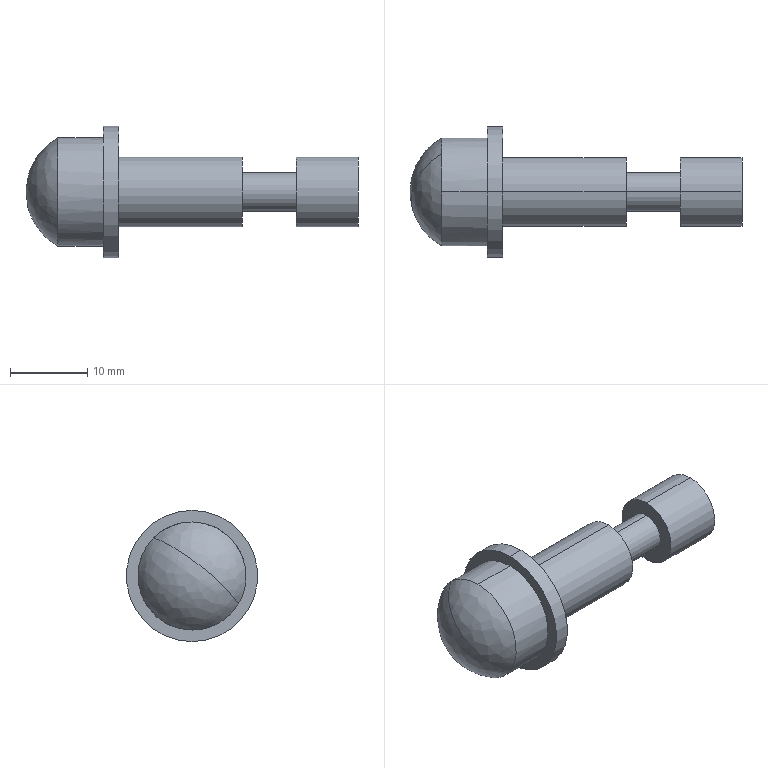Part | SolidWorks | features BaseBody 1 | 1 solid | 17 faces | box 43 x 17 x 17 mm | volume 3377 mm3 | cylinder 10 | plane 5 | spline 2 | commonest cylinder face diameters 9 x4 5 x2 14 x2 17 x2
STEP:
#1=CARTESIAN_POINT('',(867.073,-4291.009,964.907));
#2=VERTEX_POINT('',#1);
#3=CARTESIAN_POINT('',(867.073,-4295.973,966.971));
#4=VERTEX_POINT('',#3);
#5=CARTESIAN_POINT('',(867.073,-4295.973,959.971));
#6=DIRECTION('',(1.,0.,0.));
#7=DIRECTION('',(0.,0.,-1.));
#8=AXIS2_PLACEMENT_3D('',#5,#6,#7);
#9=CIRCLE('',#8,7.);
#10=EDGE_CURVE('',#2,#4,#9,.T.);
#11=ORIENTED_EDGE('',*,*,#10,.F.);
#12=CARTESIAN_POINT('',(867.073,-4301.97,956.36));
#13=VERTEX_POINT('',#12);
#14=CARTESIAN_POINT('',(870.946,-4295.973,959.971));
#15=DIRECTION('',(0.2119,-0.6009,0.7707));
#16=DIRECTION('',(0.1555,0.7993,0.5805));
#17=AXIS2_PLACEMENT_3D('',#14,#15,#16);
#18=CIRCLE('',#17,8.);
#19=EDGE_CURVE('',#2,#13,#18,.T.);
#20=ORIENTED_EDGE('',*,*,#19,.T.);
#21=CARTESIAN_POINT('',(867.073,-4295.973,959.971));
#22=DIRECTION('',(1.,0.,0.));
#23=DIRECTION('',(0.,0.,-1.));
#24=AXIS2_PLACEMENT_3D('',#21,#22,#23);
#25=CIRCLE('',#24,7.);
#26=EDGE_CURVE('',#4,#13,#25,.T.);
#27=ORIENTED_EDGE('',*,*,#26,.F.);
#28=EDGE_LOOP('',(#11,#20,#27));
#29=FACE_OUTER_BOUND('',#28,.T.);
#30=CARTESIAN_POINT('',(867.159,-4290.959,964.923));
#31=CARTESIAN_POINT('',(867.476,-4291.86,966.078));
#32=CARTESIAN_POINT('',(868.38,-4292.673,966.955));
#33=CARTESIAN_POINT('',(869.698,-4293.242,967.387));
#34=CARTESIAN_POINT('',(861.079,-4294.485,963.844));
#35=CARTESIAN_POINT('',(861.757,-4296.406,966.308));
#36=CARTESIAN_POINT('',(863.685,-4298.14,968.179));
#37=CARTESIAN_POINT('',(866.495,-4299.355,969.099));
#38=CARTESIAN_POINT('',(861.079,-4300.092,959.472));
#39=CARTESIAN_POINT('',(861.684,-4301.807,961.672));
#40=CARTESIAN_POINT('',(863.405,-4303.354,963.341));
#41=CARTESIAN_POINT('',(865.913,-4304.439,964.163));
#42=CARTESIAN_POINT('',(867.159,-4301.997,956.315));
#43=CARTESIAN_POINT('',(867.333,-4302.492,956.95));
#44=CARTESIAN_POINT('',(867.829,-4302.938,957.431));
#45=CARTESIAN_POINT('',(868.553,-4303.251,957.668));
#46=(BOUNDED_SURFACE()B_SPLINE_SURFACE(3,3,((#30,#31,#32,#33),(#34,#35,#36,#37),(#38,#39,#40,#41),(#42,#43,#44,#45)),.UNSPECIFIED.,.F.,.F.,.T.)B_SPLINE_SURFACE_WITH_KNOTS((4,4),(4,4),(0.,1.),(0.,1.),.UNSPECIFIED.)GEOMETRIC_REPRESENTATION_ITEM()RATIONAL_B_SPLINE_SURFACE(((1.,0.9364,0.9364,1.),(0.6562,0.6145,0.6145,0.6562),(0.6562,0.6145,0.6145,0.6562),(1.,0.9364,0.9364,1.)))REPRESENTATION_ITEM('')SURFACE());
#47=ADVANCED_FACE('',(#29),#46,.T.);
#48=CARTESIAN_POINT('',(874.946,-4295.973,955.471));
#49=VERTEX_POINT('',#48);
#50=CARTESIAN_POINT('',(874.946,-4295.973,964.471));
#51=VERTEX_POINT('',#50);
#52=CARTESIAN_POINT('',(874.946,-4295.973,959.971));
#53=DIRECTION('',(1.,0.,0.));
#54=DIRECTION('',(0.,0.,-1.));
#55=AXIS2_PLACEMENT_3D('',#52,#53,#54);
#56=CIRCLE('',#55,4.5);
#57=EDGE_CURVE('',#49,#51,#56,.T.);
#58=ORIENTED_EDGE('',*,*,#57,.T.);
#59=CARTESIAN_POINT('',(890.946,-4295.973,964.471));
#60=VERTEX_POINT('',#59);
#61=CARTESIAN_POINT('',(880.946,-4295.973,964.471));
#62=DIRECTION('',(1.,0.,0.));
#63=VECTOR('',#62,1000.);
#64=LINE('',#61,#63);
#65=EDGE_CURVE('',#51,#60,#64,.T.);
#66=ORIENTED_EDGE('',*,*,#65,.T.);
#67=CARTESIAN_POINT('',(890.946,-4295.973,955.471));
#68=VERTEX_POINT('',#67);
#69=CARTESIAN_POINT('',(890.946,-4295.973,959.971));
#70=DIRECTION('',(-1.,0.,0.));
#71=DIRECTION('',(0.,0.,-1.));
#72=AXIS2_PLACEMENT_3D('',#69,#70,#71);
#73=CIRCLE('',#72,4.5);
#74=EDGE_CURVE('',#60,#68,#73,.T.);
#75=ORIENTED_EDGE('',*,*,#74,.T.);
#76=CARTESIAN_POINT('',(880.946,-4295.973,955.471));
#77=DIRECTION('',(1.,0.,0.));
#78=VECTOR('',#77,1000.);
#79=LINE('',#76,#78);
#80=EDGE_CURVE('',#49,#68,#79,.T.);
#81=ORIENTED_EDGE('',*,*,#80,.F.);
#82=EDGE_LOOP('',(#58,#66,#75,#81));
#83=FACE_OUTER_BOUND('',#82,.T.);
#84=CARTESIAN_POINT('',(880.946,-4295.973,959.971));
#85=DIRECTION('',(1.,0.,0.));
#86=DIRECTION('',(0.,0.,-1.));
#87=AXIS2_PLACEMENT_3D('',#84,#85,#86);
#88=CYLINDRICAL_SURFACE('',#87,4.5);
#89=ADVANCED_FACE('',(#83),#88,.T.);
#90=CARTESIAN_POINT('',(890.946,-4295.973,962.471));
#91=VERTEX_POINT('',#90);
#92=CARTESIAN_POINT('',(890.946,-4295.973,957.471));
#93=VERTEX_POINT('',#92);
#94=CARTESIAN_POINT('',(890.946,-4295.973,959.971));
#95=DIRECTION('',(-1.,0.,0.));
#96=DIRECTION('',(0.,0.,-1.));
#97=AXIS2_PLACEMENT_3D('',#94,#95,#96);
#98=CIRCLE('',#97,2.5);
#99=EDGE_CURVE('',#91,#93,#98,.T.);
#100=ORIENTED_EDGE('',*,*,#99,.F.);
#101=CARTESIAN_POINT('',(897.946,-4295.973,962.471));
#102=VERTEX_POINT('',#101);
#103=CARTESIAN_POINT('',(892.446,-4295.973,962.471));
#104=DIRECTION('',(1.,0.,0.));
#105=VECTOR('',#104,1000.);
#106=LINE('',#103,#105);
#107=EDGE_CURVE('',#91,#102,#106,.T.);
#108=ORIENTED_EDGE('',*,*,#107,.T.);
#109=CARTESIAN_POINT('',(897.946,-4295.973,957.471));
#110=VERTEX_POINT('',#109);
#111=CARTESIAN_POINT('',(897.946,-4295.973,959.971));
#112=DIRECTION('',(-1.,0.,0.));
#113=DIRECTION('',(0.,0.,-1.));
#114=AXIS2_PLACEMENT_3D('',#111,#112,#113);
#115=CIRCLE('',#114,2.5);
#116=EDGE_CURVE('',#102,#110,#115,.T.);
#117=ORIENTED_EDGE('',*,*,#116,.T.);
#118=CARTESIAN_POINT('',(892.446,-4295.973,957.471));
#119=DIRECTION('',(1.,0.,0.));
#120=VECTOR('',#119,1000.);
#121=LINE('',#118,#120);
#122=EDGE_CURVE('',#93,#110,#121,.T.);
#123=ORIENTED_EDGE('',*,*,#122,.F.);
#124=EDGE_LOOP('',(#100,#108,#117,#123));
#125=FACE_OUTER_BOUND('',#124,.T.);
#126=CARTESIAN_POINT('',(892.446,-4295.973,959.971));
#127=DIRECTION('',(1.,0.,0.));
#128=DIRECTION('',(0.,0.,-1.));
#129=AXIS2_PLACEMENT_3D('',#126,#127,#128);
#130=CYLINDRICAL_SURFACE('',#129,2.5);
#131=ADVANCED_FACE('',(#125),#130,.T.);
#132=CARTESIAN_POINT('',(872.946,-4295.973,951.471));
#133=VERTEX_POINT('',#132);
#134=CARTESIAN_POINT('',(872.946,-4295.973,968.471));
#135=VERTEX_POINT('',#134);
#136=CARTESIAN_POINT('',(872.946,-4295.973,959.971));
#137=DIRECTION('',(1.,0.,0.));
#138=DIRECTION('',(0.,0.,-1.));
#139=AXIS2_PLACEMENT_3D('',#136,#137,#138);
#140=CIRCLE('',#139,8.5);
#141=EDGE_CURVE('',#133,#135,#140,.T.);
#142=ORIENTED_EDGE('',*,*,#141,.T.);
#143=CARTESIAN_POINT('',(874.946,-4295.973,968.471));
#144=VERTEX_POINT('',#143);
#145=CARTESIAN_POINT('',(871.946,-4295.973,968.471));
#146=DIRECTION('',(1.,0.,0.));
#147=VECTOR('',#146,1000.);
#148=LINE('',#145,#147);
#149=EDGE_CURVE('',#135,#144,#148,.T.);
#150=ORIENTED_EDGE('',*,*,#149,.T.);
#151=CARTESIAN_POINT('',(874.946,-4295.973,951.471));
#152=VERTEX_POINT('',#151);
#153=CARTESIAN_POINT('',(874.946,-4295.973,959.971));
#154=DIRECTION('',(1.,0.,0.));
#155=DIRECTION('',(0.,0.,-1.));
#156=AXIS2_PLACEMENT_3D('',#153,#154,#155);
#157=CIRCLE('',#156,8.5);
#158=EDGE_CURVE('',#152,#144,#157,.T.);
#159=ORIENTED_EDGE('',*,*,#158,.F.);
#160=CARTESIAN_POINT('',(871.946,-4295.973,951.471));
#161=DIRECTION('',(1.,0.,0.));
#162=VECTOR('',#161,1000.);
#163=LINE('',#160,#162);
#164=EDGE_CURVE('',#133,#152,#163,.T.);
#165=ORIENTED_EDGE('',*,*,#164,.F.);
#166=EDGE_LOOP('',(#142,#150,#159,#165));
#167=FACE_OUTER_BOUND('',#166,.T.);
#168=CARTESIAN_POINT('',(871.946,-4295.973,959.971));
#169=DIRECTION('',(1.,0.,0.));
#170=DIRECTION('',(0.,0.,-1.));
#171=AXIS2_PLACEMENT_3D('',#168,#169,#170);
#172=CYLINDRICAL_SURFACE('',#171,8.5);
#173=ADVANCED_FACE('',(#167),#172,.T.);
#174=CARTESIAN_POINT('',(897.946,-4295.973,964.471));
#175=VERTEX_POINT('',#174);
#176=CARTESIAN_POINT('',(897.946,-4295.973,955.471));
#177=VERTEX_POINT('',#176);
#178=CARTESIAN_POINT('',(897.946,-4295.973,959.971));
#179=DIRECTION('',(-1.,0.,0.));
#180=DIRECTION('',(0.,0.,-1.));
#181=AXIS2_PLACEMENT_3D('',#178,#179,#180);
#182=CIRCLE('',#181,4.5);
#183=EDGE_CURVE('',#175,#177,#182,.T.);
#184=ORIENTED_EDGE('',*,*,#183,.F.);
#185=CARTESIAN_POINT('',(905.946,-4295.973,964.471));
#186=VERTEX_POINT('',#185);
#187=CARTESIAN_POINT('',(899.946,-4295.973,964.471));
#188=DIRECTION('',(1.,0.,0.));
#189=VECTOR('',#188,1000.);
#190=LINE('',#187,#189);
#191=EDGE_CURVE('',#175,#186,#190,.T.);
#192=ORIENTED_EDGE('',*,*,#191,.T.);
#193=CARTESIAN_POINT('',(905.946,-4295.973,955.471));
#194=VERTEX_POINT('',#193);
#195=CARTESIAN_POINT('',(905.946,-4295.973,959.971));
#196=DIRECTION('',(-1.,0.,0.));
#197=DIRECTION('',(0.,0.,-1.));
#198=AXIS2_PLACEMENT_3D('',#195,#196,#197);
#199=CIRCLE('',#198,4.5);
#200=EDGE_CURVE('',#186,#194,#199,.T.);
#201=ORIENTED_EDGE('',*,*,#200,.T.);
#202=CARTESIAN_POINT('',(899.946,-4295.973,955.471));
#203=DIRECTION('',(1.,0.,0.));
#204=VECTOR('',#203,1000.);
#205=LINE('',#202,#204);
#206=EDGE_CURVE('',#177,#194,#205,.T.);
#207=ORIENTED_EDGE('',*,*,#206,.F.);
#208=EDGE_LOOP('',(#184,#192,#201,#207));
#209=FACE_OUTER_BOUND('',#208,.T.);
#210=CARTESIAN_POINT('',(899.946,-4295.973,959.971));
#211=DIRECTION('',(1.,0.,0.));
#212=DIRECTION('',(0.,0.,-1.));
#213=AXIS2_PLACEMENT_3D('',#210,#211,#212);
#214=CYLINDRICAL_SURFACE('',#213,4.5);
#215=ADVANCED_FACE('',(#209),#214,.T.);
#216=CARTESIAN_POINT('',(867.073,-4295.973,952.971));
#217=VERTEX_POINT('',#216);
#218=CARTESIAN_POINT('',(867.073,-4295.973,959.971));
#219=DIRECTION('',(1.,0.,0.));
#220=DIRECTION('',(0.,0.,-1.));
#221=AXIS2_PLACEMENT_3D('',#218,#219,#220);
#222=CIRCLE('',#221,7.);
#223=EDGE_CURVE('',#217,#2,#222,.T.);
#224=ORIENTED_EDGE('',*,*,#223,.T.);
#225=ORIENTED_EDGE('',*,*,#10,.T.);
#226=CARTESIAN_POINT('',(872.946,-4295.973,966.971));
#227=VERTEX_POINT('',#226);
#228=CARTESIAN_POINT('',(869.009,-4295.973,966.971));
#229=DIRECTION('',(1.,0.,0.));
#230=VECTOR('',#229,1000.);
#231=LINE('',#228,#230);
#232=EDGE_CURVE('',#4,#227,#231,.T.);
#233=ORIENTED_EDGE('',*,*,#232,.T.);
#234=CARTESIAN_POINT('',(872.946,-4295.973,952.971));
#235=VERTEX_POINT('',#234);
#236=CARTESIAN_POINT('',(872.946,-4295.973,959.971));
#237=DIRECTION('',(1.,0.,0.));
#238=DIRECTION('',(0.,0.,-1.));
#239=AXIS2_PLACEMENT_3D('',#236,#237,#238);
#240=CIRCLE('',#239,7.);
#241=EDGE_CURVE('',#235,#227,#240,.T.);
#242=ORIENTED_EDGE('',*,*,#241,.F.);
#243=CARTESIAN_POINT('',(869.009,-4295.973,952.971));
#244=DIRECTION('',(1.,0.,0.));
#245=VECTOR('',#244,1000.);
#246=LINE('',#243,#245);
#247=EDGE_CURVE('',#217,#235,#246,.T.);
#248=ORIENTED_EDGE('',*,*,#247,.F.);
#249=EDGE_LOOP('',(#224,#225,#233,#242,#248));
#250=FACE_OUTER_BOUND('',#249,.T.);
#251=CARTESIAN_POINT('',(869.009,-4295.973,959.971));
#252=DIRECTION('',(1.,0.,0.));
#253=DIRECTION('',(0.,0.,-1.));
#254=AXIS2_PLACEMENT_3D('',#251,#252,#253);
#255=CYLINDRICAL_SURFACE('',#254,7.);
#256=ADVANCED_FACE('',(#250),#255,.T.);
#257=ORIENTED_EDGE('',*,*,#65,.F.);
#258=CARTESIAN_POINT('',(874.946,-4295.973,959.971));
#259=DIRECTION('',(1.,0.,0.));
#260=DIRECTION('',(0.,0.,-1.));
#261=AXIS2_PLACEMENT_3D('',#258,#259,#260);
#262=CIRCLE('',#261,4.5);
#263=EDGE_CURVE('',#51,#49,#262,.T.);
#264=ORIENTED_EDGE('',*,*,#263,.T.);
#265=ORIENTED_EDGE('',*,*,#80,.T.);
#266=CARTESIAN_POINT('',(890.946,-4295.973,959.971));
#267=DIRECTION('',(-1.,0.,0.));
#268=DIRECTION('',(0.,0.,-1.));
#269=AXIS2_PLACEMENT_3D('',#266,#267,#268);
#270=CIRCLE('',#269,4.5);
#271=EDGE_CURVE('',#68,#60,#270,.T.);
#272=ORIENTED_EDGE('',*,*,#271,.T.);
#273=EDGE_LOOP('',(#257,#264,#265,#272));
#274=FACE_OUTER_BOUND('',#273,.T.);
#275=CARTESIAN_POINT('',(880.946,-4295.973,959.971));
#276=DIRECTION('',(1.,0.,0.));
#277=DIRECTION('',(0.,0.,-1.));
#278=AXIS2_PLACEMENT_3D('',#275,#276,#277);
#279=CYLINDRICAL_SURFACE('',#278,4.5);
#280=ADVANCED_FACE('',(#274),#279,.T.);
#281=ORIENTED_EDGE('',*,*,#271,.F.);
#282=ORIENTED_EDGE('',*,*,#74,.F.);
#283=EDGE_LOOP('',(#281,#282));
#284=FACE_OUTER_BOUND('',#283,.T.);
#285=CARTESIAN_POINT('',(890.946,-4295.973,959.971));
#286=DIRECTION('',(-1.,0.,0.));
#287=DIRECTION('',(0.,0.,-1.));
#288=AXIS2_PLACEMENT_3D('',#285,#286,#287);
#289=CIRCLE('',#288,2.5);
#290=EDGE_CURVE('',#93,#91,#289,.T.);
#291=ORIENTED_EDGE('',*,*,#290,.T.);
#292=ORIENTED_EDGE('',*,*,#99,.T.);
#293=EDGE_LOOP('',(#291,#292));
#294=FACE_BOUND('',#293,.T.);
#295=CARTESIAN_POINT('',(890.946,-4292.473,959.971));
#296=DIRECTION('',(1.,0.,0.));
#297=DIRECTION('',(0.,0.,-1.));
#298=AXIS2_PLACEMENT_3D('',#295,#296,#297);
#299=PLANE('',#298);
#300=ADVANCED_FACE('',(#284,#294),#299,.T.);
#301=ORIENTED_EDGE('',*,*,#158,.T.);
#302=CARTESIAN_POINT('',(874.946,-4295.973,959.971));
#303=DIRECTION('',(1.,0.,0.));
#304=DIRECTION('',(0.,0.,-1.));
#305=AXIS2_PLACEMENT_3D('',#302,#303,#304);
#306=CIRCLE('',#305,8.5);
#307=EDGE_CURVE('',#144,#152,#306,.T.);
#308=ORIENTED_EDGE('',*,*,#307,.T.);
#309=EDGE_LOOP('',(#301,#308));
#310=FACE_OUTER_BOUND('',#309,.T.);
#311=ORIENTED_EDGE('',*,*,#57,.F.);
#312=ORIENTED_EDGE('',*,*,#263,.F.);
#313=EDGE_LOOP('',(#311,#312));
#314=FACE_BOUND('',#313,.T.);
#315=CARTESIAN_POINT('',(874.946,-4289.473,959.971));
#316=DIRECTION('',(1.,0.,0.));
#317=DIRECTION('',(0.,0.,-1.));
#318=AXIS2_PLACEMENT_3D('',#315,#316,#317);
#319=PLANE('',#318);
#320=ADVANCED_FACE('',(#310,#314),#319,.T.);
#321=ORIENTED_EDGE('',*,*,#107,.F.);
#322=ORIENTED_EDGE('',*,*,#290,.F.);
#323=ORIENTED_EDGE('',*,*,#122,.T.);
#324=CARTESIAN_POINT('',(897.946,-4295.973,959.971));
#325=DIRECTION('',(-1.,0.,0.));
#326=DIRECTION('',(0.,0.,-1.));
#327=AXIS2_PLACEMENT_3D('',#324,#325,#326);
#328=CIRCLE('',#327,2.5);
#329=EDGE_CURVE('',#110,#102,#328,.T.);
#330=ORIENTED_EDGE('',*,*,#329,.T.);
#331=EDGE_LOOP('',(#321,#322,#323,#330));
#332=FACE_OUTER_BOUND('',#331,.T.);
#333=CARTESIAN_POINT('',(892.446,-4295.973,959.971));
#334=DIRECTION('',(1.,0.,0.));
#335=DIRECTION('',(0.,0.,-1.));
#336=AXIS2_PLACEMENT_3D('',#333,#334,#335);
#337=CYLINDRICAL_SURFACE('',#336,2.5);
#338=ADVANCED_FACE('',(#332),#337,.T.);
#339=ORIENTED_EDGE('',*,*,#149,.F.);
#340=CARTESIAN_POINT('',(872.946,-4295.973,959.971));
#341=DIRECTION('',(1.,0.,0.));
#342=DIRECTION('',(0.,0.,-1.));
#343=AXIS2_PLACEMENT_3D('',#340,#341,#342);
#344=CIRCLE('',#343,8.5);
#345=EDGE_CURVE('',#135,#133,#344,.T.);
#346=ORIENTED_EDGE('',*,*,#345,.T.);
#347=ORIENTED_EDGE('',*,*,#164,.T.);
#348=ORIENTED_EDGE('',*,*,#307,.F.);
#349=EDGE_LOOP('',(#339,#346,#347,#348));
#350=FACE_OUTER_BOUND('',#349,.T.);
#351=CARTESIAN_POINT('',(871.946,-4295.973,959.971));
#352=DIRECTION('',(1.,0.,0.));
#353=DIRECTION('',(0.,0.,-1.));
#354=AXIS2_PLACEMENT_3D('',#351,#352,#353);
#355=CYLINDRICAL_SURFACE('',#354,8.5);
#356=ADVANCED_FACE('',(#350),#355,.T.);
#357=ORIENTED_EDGE('',*,*,#329,.F.);
#358=ORIENTED_EDGE('',*,*,#116,.F.);
#359=EDGE_LOOP('',(#357,#358));
#360=FACE_BOUND('',#359,.T.);
#361=CARTESIAN_POINT('',(897.946,-4295.973,959.971));
#362=DIRECTION('',(-1.,0.,0.));
#363=DIRECTION('',(0.,0.,-1.));
#364=AXIS2_PLACEMENT_3D('',#361,#362,#363);
#365=CIRCLE('',#364,4.5);
#366=EDGE_CURVE('',#177,#175,#365,.T.);
#367=ORIENTED_EDGE('',*,*,#366,.T.);
#368=ORIENTED_EDGE('',*,*,#183,.T.);
#369=EDGE_LOOP('',(#367,#368));
#370=FACE_OUTER_BOUND('',#369,.T.);
#371=CARTESIAN_POINT('',(897.946,-4292.473,959.971));
#372=DIRECTION('',(-1.,0.,0.));
#373=DIRECTION('',(0.,0.,1.));
#374=AXIS2_PLACEMENT_3D('',#371,#372,#373);
#375=PLANE('',#374);
#376=ADVANCED_FACE('',(#360,#370),#375,.T.);
#377=ORIENTED_EDGE('',*,*,#241,.T.);
#378=CARTESIAN_POINT('',(872.946,-4295.973,959.971));
#379=DIRECTION('',(1.,0.,0.));
#380=DIRECTION('',(0.,0.,-1.));
#381=AXIS2_PLACEMENT_3D('',#378,#379,#380);
#382=CIRCLE('',#381,7.);
#383=EDGE_CURVE('',#227,#235,#382,.T.);
#384=ORIENTED_EDGE('',*,*,#383,.T.);
#385=EDGE_LOOP('',(#377,#384));
#386=FACE_BOUND('',#385,.T.);
#387=ORIENTED_EDGE('',*,*,#141,.F.);
#388=ORIENTED_EDGE('',*,*,#345,.F.);
#389=EDGE_LOOP('',(#387,#388));
#390=FACE_OUTER_BOUND('',#389,.T.);
#391=CARTESIAN_POINT('',(872.946,-4288.223,959.971));
#392=DIRECTION('',(-1.,0.,0.));
#393=DIRECTION('',(0.,0.,1.));
#394=AXIS2_PLACEMENT_3D('',#391,#392,#393);
#395=PLANE('',#394);
#396=ADVANCED_FACE('',(#386,#390),#395,.T.);
#397=ORIENTED_EDGE('',*,*,#191,.F.);
#398=ORIENTED_EDGE('',*,*,#366,.F.);
#399=ORIENTED_EDGE('',*,*,#206,.T.);
#400=CARTESIAN_POINT('',(905.946,-4295.973,959.971));
#401=DIRECTION('',(-1.,0.,0.));
#402=DIRECTION('',(0.,0.,-1.));
#403=AXIS2_PLACEMENT_3D('',#400,#401,#402);
#404=CIRCLE('',#403,4.5);
#405=EDGE_CURVE('',#194,#186,#404,.T.);
#406=ORIENTED_EDGE('',*,*,#405,.T.);
#407=EDGE_LOOP('',(#397,#398,#399,#406));
#408=FACE_OUTER_BOUND('',#407,.T.);
#409=CARTESIAN_POINT('',(899.946,-4295.973,959.971));
#410=DIRECTION('',(1.,0.,0.));
#411=DIRECTION('',(0.,0.,-1.));
#412=AXIS2_PLACEMENT_3D('',#409,#410,#411);
#413=CYLINDRICAL_SURFACE('',#412,4.5);
#414=ADVANCED_FACE('',(#408),#413,.T.);
#415=ORIENTED_EDGE('',*,*,#232,.F.);
#416=ORIENTED_EDGE('',*,*,#26,.T.);
#417=CARTESIAN_POINT('',(867.073,-4295.973,959.971));
#418=DIRECTION('',(1.,0.,0.));
#419=DIRECTION('',(0.,0.,-1.));
#420=AXIS2_PLACEMENT_3D('',#417,#418,#419);
#421=CIRCLE('',#420,7.);
#422=EDGE_CURVE('',#13,#217,#421,.T.);
#423=ORIENTED_EDGE('',*,*,#422,.T.);
#424=ORIENTED_EDGE('',*,*,#247,.T.);
#425=ORIENTED_EDGE('',*,*,#383,.F.);
#426=EDGE_LOOP('',(#415,#416,#423,#424,#425));
#427=FACE_OUTER_BOUND('',#426,.T.);
#428=CARTESIAN_POINT('',(869.009,-4295.973,959.971));
#429=DIRECTION('',(1.,0.,0.));
#430=DIRECTION('',(0.,0.,-1.));
#431=AXIS2_PLACEMENT_3D('',#428,#429,#430);
#432=CYLINDRICAL_SURFACE('',#431,7.);
#433=ADVANCED_FACE('',(#427),#432,.T.);
#434=ORIENTED_EDGE('',*,*,#405,.F.);
#435=ORIENTED_EDGE('',*,*,#200,.F.);
#436=EDGE_LOOP('',(#434,#435));
#437=FACE_OUTER_BOUND('',#436,.T.);
#438=CARTESIAN_POINT('',(905.946,-4293.723,959.971));
#439=DIRECTION('',(1.,0.,0.));
#440=DIRECTION('',(0.,0.,-1.));
#441=AXIS2_PLACEMENT_3D('',#438,#439,#440);
#442=PLANE('',#441);
#443=ADVANCED_FACE('',(#437),#442,.T.);
#444=ORIENTED_EDGE('',*,*,#19,.F.);
#445=ORIENTED_EDGE('',*,*,#223,.F.);
#446=ORIENTED_EDGE('',*,*,#422,.F.);
#447=EDGE_LOOP('',(#444,#445,#446));
#448=FACE_OUTER_BOUND('',#447,.T.);
#449=CARTESIAN_POINT('',(869.796,-4288.071,960.449));
#450=CARTESIAN_POINT('',(867.806,-4288.421,961.465));
#451=CARTESIAN_POINT('',(866.852,-4289.502,963.208));
#452=CARTESIAN_POINT('',(867.331,-4290.861,964.951));
#453=CARTESIAN_POINT('',(866.481,-4288.159,953.929));
#454=CARTESIAN_POINT('',(862.05,-4288.94,956.192));
#455=CARTESIAN_POINT('',(859.925,-4291.346,960.074));
#456=CARTESIAN_POINT('',(860.992,-4294.373,963.956));
#457=CARTESIAN_POINT('',(865.863,-4294.589,950.497));
#458=CARTESIAN_POINT('',(861.9,-4295.288,952.521));
#459=CARTESIAN_POINT('',(859.999,-4297.439,955.993));
#460=CARTESIAN_POINT('',(860.954,-4300.146,959.465));
#461=CARTESIAN_POINT('',(868.6,-4300.508,953.812));
#462=CARTESIAN_POINT('',(867.516,-4300.699,954.366));
#463=CARTESIAN_POINT('',(866.996,-4301.287,955.315));
#464=CARTESIAN_POINT('',(867.257,-4302.028,956.265));
#465=(BOUNDED_SURFACE()B_SPLINE_SURFACE(3,3,((#449,#450,#451,#452),(#453,#454,#455,#456),(#457,#458,#459,#460),(#461,#462,#463,#464)),.UNSPECIFIED.,.F.,.F.,.F.)B_SPLINE_SURFACE_WITH_KNOTS((4,4),(4,4),(0.,1.),(0.,1.),.UNSPECIFIED.)GEOMETRIC_REPRESENTATION_ITEM()RATIONAL_B_SPLINE_SURFACE(((1.,0.861,0.861,1.),(0.6447,0.5551,0.5551,0.6447),(0.6447,0.5551,0.5551,0.6447),(1.,0.861,0.861,1.)))REPRESENTATION_ITEM('')SURFACE());
#466=ADVANCED_FACE('',(#448),#465,.T.);
#467=CLOSED_SHELL('',(#47,#89,#131,#173,#215,#256,#280,#300,#320,#338,#356,#376,#396,#414,#433,#443,#466));
#468=MANIFOLD_SOLID_BREP('',#467);
#469=CARTESIAN_POINT('',(0.,0.,0.));
#470=DIRECTION('',(0.,0.,1.));
#471=DIRECTION('',(1.,0.,0.));
#472=AXIS2_PLACEMENT_3D('',#469,#470,#471);
#473=(LENGTH_UNIT()NAMED_UNIT(*)SI_UNIT(.MILLI.,.METRE.));
#474=UNCERTAINTY_MEASURE_WITH_UNIT(LENGTH_MEASURE(0.00001),#473,'','');
#475=(NAMED_UNIT(*)PLANE_ANGLE_UNIT()SI_UNIT($,.RADIAN.));
#476=(NAMED_UNIT(*)SI_UNIT($,.STERADIAN.)SOLID_ANGLE_UNIT());
#477=(GEOMETRIC_REPRESENTATION_CONTEXT(3)GLOBAL_UNCERTAINTY_ASSIGNED_CONTEXT((#474))GLOBAL_UNIT_ASSIGNED_CONTEXT((#473,#475,#476))REPRESENTATION_CONTEXT('',''));
#478=ADVANCED_BREP_SHAPE_REPRESENTATION('',(#468,#472),#477);